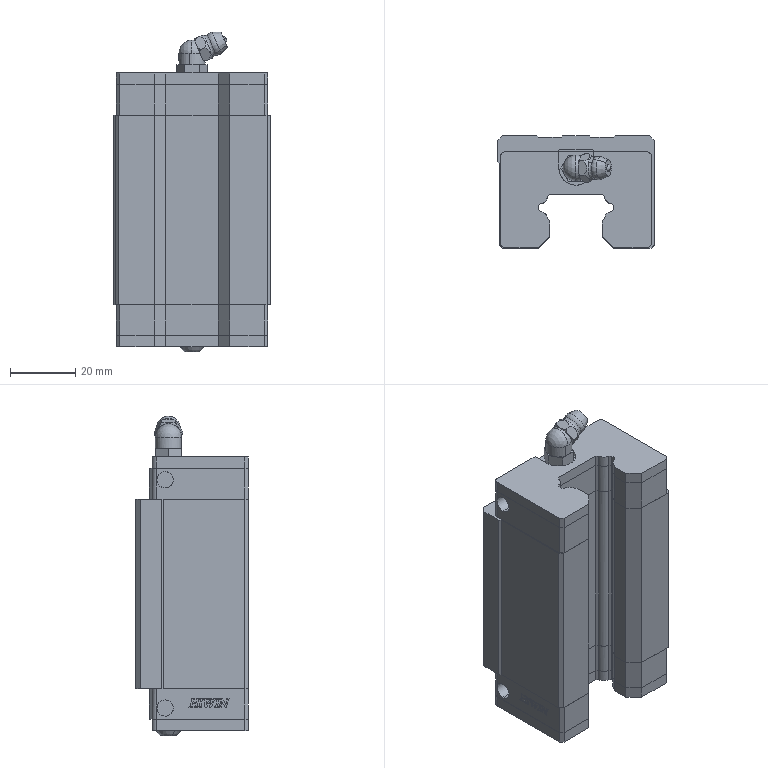Part | NX | features BREP 7 | 7 solids | 571 faces | box 48 x 34.5 x 98 mm | volume 103942 mm3 | plane 406 | cylinder 136 | cone 16 | torus 7 | sphere 4 | spline 2 | commonest cylinder face diameters 4.6 x20 0.207 x17 0.24 x17 6 x12 0.104 x9 0.12 x9